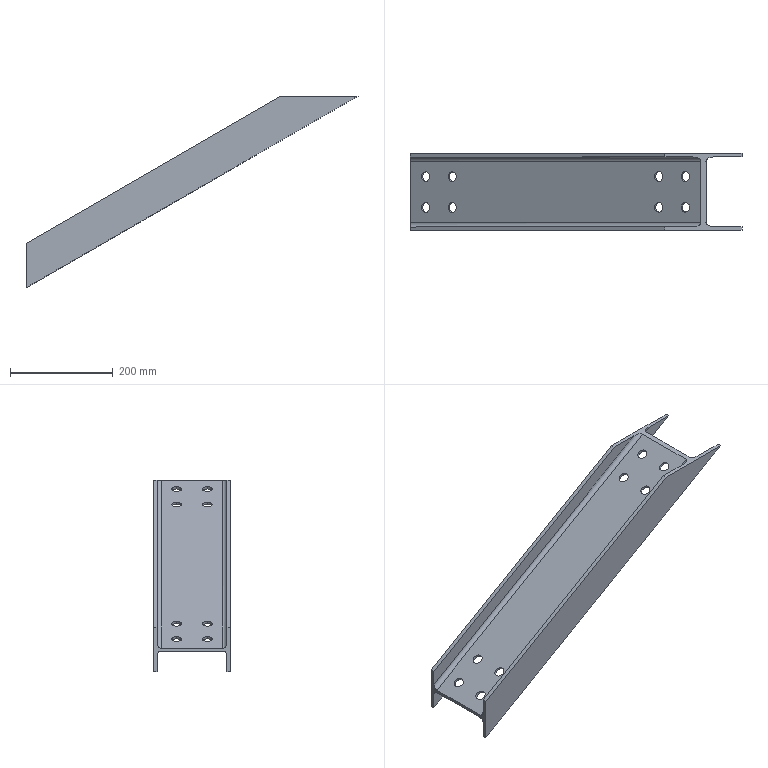Part | STEP file | 粉仓Diagonal Brace梁6-2_Default<As Machined> | 1 solid | 34 faces | box 646.577 x 150 x 373.301 mm | volume 1166718 mm3 | cylinder 20 | plane 14 | commonest cylinder face diameters 19 x16 16 x4